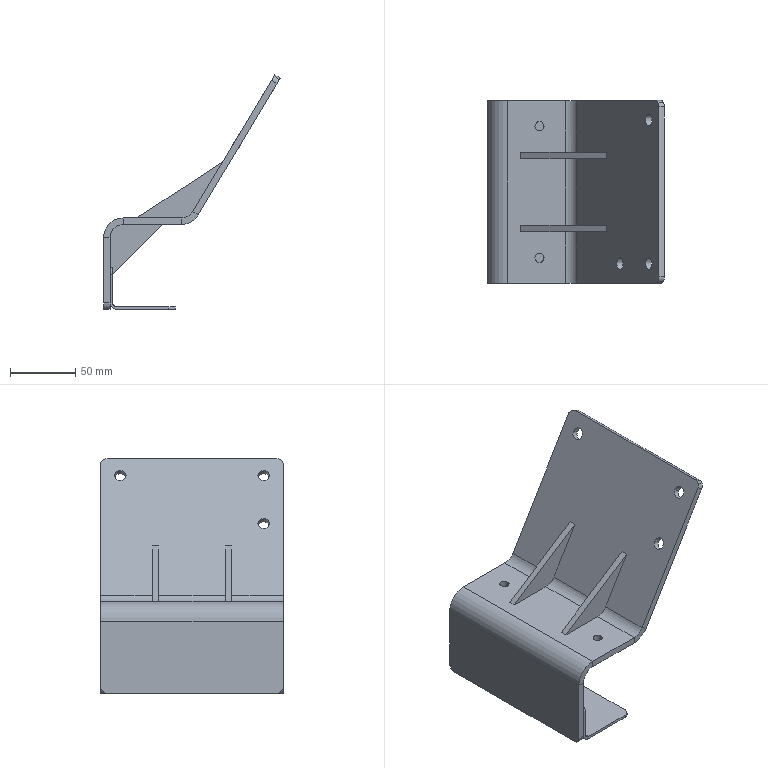Part | NX | features BREP 2 | 2 solids | 88 faces | box 135.55 x 140 x 179.776 mm | volume 207099 mm3 | cylinder 44 | plane 44 | commonest cylinder face diameters 10 x16 20 x9 7 x8 9 x6 30 x3 6 x2